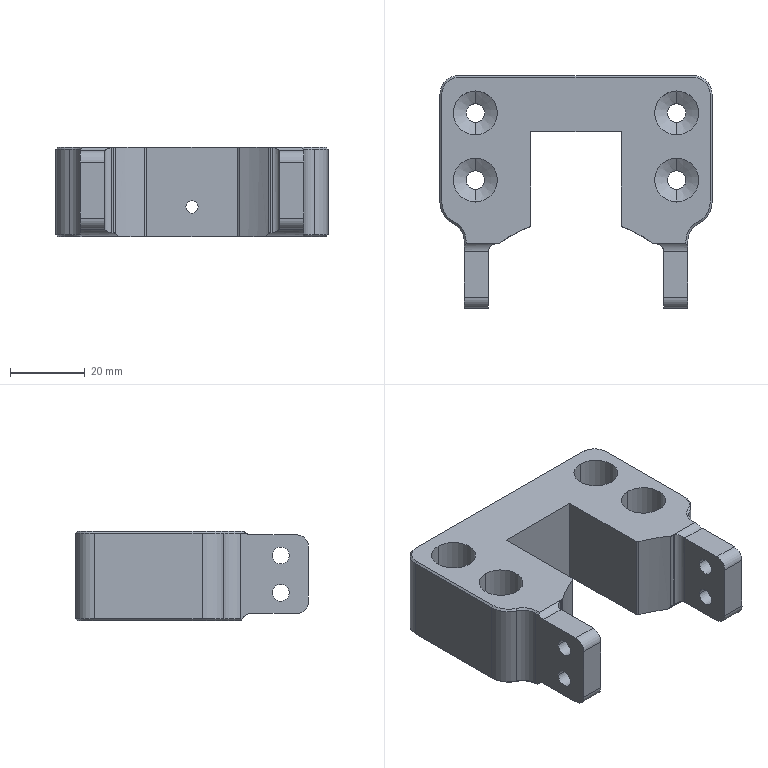NC program | NX | posted with a generic post | part box 73 x 62.4 x 24 mm
Lines 2249 to 2496 of 2496:
(ZLEVEL_PROFILE_1_COPY_1_COPY_COPY_1_COPY_COPY , TOOL : D6A45)
N4454 T07 M6
N4456 G54
N4458 G17 G0 G90 X27.544 Y21.2 S7500 M3
N4460 G43 Z30. H7
N4462 Z1.
N4464 G94 G1 Z-2. F1000.
N4466 G3 X26.999 Y21.744 R0.544
N4468 X27.544 Y21.2 R-0.544
N4470 X27.394 Y21.46 R0.3
N4472 G1 Z-1.
N4474 G0 Z30.
N4476 X-27.544 Y21.2
N4478 Z1.
N4480 G1 Z-2.
N4482 Y21.199
N4484 G3 X-26.999 Y20.656 R0.544
N4486 X-27.544 Y21.2 R-0.544
N4488 X-27.394 Y20.94 R0.3
N4490 G1 Z-1.
N4492 G0 Z30.
N4494 X27.544 Y3.2
N4496 Z1.
N4498 G1 Z-2.
N4500 G3 X27. Y3.744 R0.544
N4502 X27.544 Y3.2 R-0.544
N4504 X27.394 Y3.46 R0.3
N4506 G1 Z-1.
N4508 G0 Z30.
N4510 X-27.544 Y3.2
N4512 Z1.
N4514 G1 Z-2.
N4516 G3 X-27. Y2.656 R0.544
N4518 X-27.544 Y3.2 R-0.544
N4520 X-27.394 Y2.94 R0.3
N4522 G1 Z-1.
N4524 G0 Z30.
N4526 X-32.48 Y-14.397
N4528 Z-1.
N4530 G1 Z-2.
N4532 X-31.756 Y-13.979
N4534 G3 X-31.456 Y-13.459 R0.6
N4536 G1 Y-13.056
N4538 G3 X-33.459 Y-9.865 R3.544
N4540 G2 X-37.956 Y-2.7 R7.956
N4542 G1 Y26.2
N4544 G2 X-31.5 Y32.656 R6.456
N4546 G1 X31.5
N4548 G2 X37.956 Y26.2 R6.456
N4550 G1 Y-2.7
N4552 G2 X33.459 Y-9.865 R7.956
N4554 G3 X31.456 Y-13.056 R3.544
N4556 G1 Y-13.459
N4558 G3 X31.756 Y-13.979 R0.6
N4560 G1 X32.478 Y-14.395
N4562 Z-1.
N4564 G0 Z30.
N4566 X18.921 Y-16.249
N4568 Z-1.
N4570 G1 Z-2.
N4572 X18.987 Y-15.384
N4574 G3 X18.727 Y-14.843 R0.6
N4576 X11.937 Y-11.277 R33.194
N4578 G2 X10.346 Y-9.82 R2.956
N4580 X10.144 Y-8.955 R1.966
N4582 G1 Y14.244
N4584 X-10.144
N4586 Y-8.955
N4588 G2 X-10.339 Y-9.806 R1.954
N4590 X-11.937 Y-11.277 R2.956
N4592 G3 X-18.727 Y-14.843 R33.194
N4594 X-18.987 Y-15.384 R0.6
N4596 G1 X-18.921 Y-16.249
N4598 Z-1.
N4600 G0 Z30.
(ZLEVEL_PROFILE_1_COPY_1_COPY_COPY_1_COPY_COPY_COPY , TOOL : D6A45)
N4602 X21.438 Y-29.185
N4604 Z-2.
N4606 G1 Z-3.
N4608 X22.241 Y-28.721
N4610 G3 X22.541 Y-28.201 R0.6
N4612 G1 Y-16.42
N4614 G3 X22.022 Y-16.72 R0.6
N4616 G1 X21.341 Y-17.899
N4618 Z-2.
N4620 G0 Z30.
N4622 X32.159 Y-16.553
N4624 Z-2.
N4626 G1 Z-3.
N4628 X30.999 Y-16.007
N4630 X30.967 Y-16.051
N4632 X30.953 Y-16.103
N4634 X30.959 Y-16.157
N4636 Y-28.202
N4638 G3 X31.259 Y-28.721 R0.6
N4640 G1 X32.063 Y-29.186
N4642 Z-2.
N4644 G0 Z30.
N4646 X-32.062 Y-29.185
N4648 Z-2.
N4650 G1 Z-3.
N4652 X-31.259 Y-28.721
N4654 G3 X-30.959 Y-28.201 R0.6
N4656 G1 Y-16.158
N4658 X-30.953 Y-16.104
N4660 X-30.967 Y-16.052
N4662 X-30.999 Y-16.008
N4664 X-32.159 Y-16.552
N4666 Z-2.
N4668 G0 Z30.
N4670 X-21.341 Y-17.899
N4672 Z-2.
N4674 G1 Z-3.
N4676 X-22.022 Y-16.72
N4678 G3 X-22.541 Y-16.42 R0.6
N4680 G1 Y-28.202
N4682 G3 X-22.241 Y-28.721 R0.6
N4684 G1 X-21.437 Y-29.186
N4686 Z-2.
N4688 G0 Z30.
(ZLEVEL_PROFILE_1_COPY_1_COPY_COPY_1_COPY_COPY_COPY_1 , TOOL : D6A45)
N4690 G55
N4692 X27.544 Y21.2
N4694 Z1.
N4696 G1 Z-2.
N4698 G3 X26.999 Y21.744 R0.544
N4700 X27.544 Y21.2 R-0.544
N4702 X27.394 Y21.46 R0.3
N4704 G1 Z-1.
N4706 G0 Z30.
N4708 X-27.544 Y21.2
N4710 Z1.
N4712 G1 Z-2.
N4714 Y21.199
N4716 G3 X-26.999 Y20.656 R0.544
N4718 X-27.544 Y21.2 R-0.544
N4720 X-27.394 Y20.94 R0.3
N4722 G1 Z-1.
N4724 G0 Z30.
N4726 X27.544 Y3.2
N4728 Z1.
N4730 G1 Z-2.
N4732 G3 X27. Y3.744 R0.544
N4734 X27.544 Y3.2 R-0.544
N4736 X27.394 Y3.46 R0.3
N4738 G1 Z-1.
N4740 G0 Z30.
N4742 X-27.544 Y3.2
N4744 Z1.
N4746 G1 Z-2.
N4748 G3 X-27. Y2.656 R0.544
N4750 X-27.544 Y3.2 R-0.544
N4752 X-27.394 Y2.94 R0.3
N4754 G1 Z-1.
N4756 G0 Z30.
N4758 X-32.48 Y-14.397
N4760 Z-1.
N4762 G1 Z-2.
N4764 X-31.756 Y-13.979
N4766 G3 X-31.456 Y-13.459 R0.6
N4768 G1 Y-13.056
N4770 G3 X-33.459 Y-9.865 R3.544
N4772 G2 X-37.956 Y-2.7 R7.956
N4774 G1 Y26.2
N4776 G2 X-31.5 Y32.656 R6.456
N4778 G1 X31.5
N4780 G2 X37.956 Y26.2 R6.456
N4782 G1 Y-2.7
N4784 G2 X33.459 Y-9.865 R7.956
N4786 G3 X31.456 Y-13.056 R3.544
N4788 G1 Y-13.459
N4790 G3 X31.756 Y-13.979 R0.6
N4792 G1 X32.478 Y-14.395
N4794 Z-1.
N4796 G0 Z30.
N4798 X18.921 Y-16.249
N4800 Z-1.
N4802 G1 Z-2.
N4804 X18.987 Y-15.384
N4806 G3 X18.727 Y-14.843 R0.6
N4808 X11.937 Y-11.277 R33.194
N4810 G2 X10.346 Y-9.82 R2.956
N4812 X10.144 Y-8.955 R1.966
N4814 G1 Y14.244
N4816 X-10.144
N4818 Y-8.955
N4820 G2 X-10.339 Y-9.806 R1.954
N4822 X-11.937 Y-11.277 R2.956
N4824 G3 X-18.727 Y-14.843 R33.194
N4826 X-18.987 Y-15.384 R0.6
N4828 G1 X-18.921 Y-16.249
N4830 Z-1.
N4832 G0 Z30.
(ZLEVEL_PROFILE_1_COPY_1_COPY_COPY_1_COPY_COPY_COPY_COPY , TOOL : D6A45)
N4834 X21.438 Y-29.185
N4836 Z-2.
N4838 G1 Z-3.
N4840 X22.241 Y-28.721
N4842 G3 X22.541 Y-28.201 R0.6
N4844 G1 Y-16.42
N4846 G3 X22.022 Y-16.72 R0.6
N4848 G1 X21.341 Y-17.899
N4850 Z-2.
N4852 G0 Z30.
N4854 X32.159 Y-16.553
N4856 Z-2.
N4858 G1 Z-3.
N4860 X30.999 Y-16.007
N4862 X30.967 Y-16.051
N4864 X30.953 Y-16.103
N4866 X30.959 Y-16.157
N4868 Y-28.202
N4870 G3 X31.259 Y-28.721 R0.6
N4872 G1 X32.063 Y-29.186
N4874 Z-2.
N4876 G0 Z30.
N4878 X-32.062 Y-29.185
N4880 Z-2.
N4882 G1 Z-3.
N4884 X-31.259 Y-28.721
N4886 G3 X-30.959 Y-28.201 R0.6
N4888 G1 Y-16.158
N4890 X-30.953 Y-16.104
N4892 X-30.967 Y-16.052
N4894 X-30.999 Y-16.008
N4896 X-32.159 Y-16.552
N4898 Z-2.
N4900 G0 Z30.
N4902 X-21.341 Y-17.899
N4904 Z-2.
N4906 G1 Z-3.
N4908 X-22.022 Y-16.72
N4910 G3 X-22.541 Y-16.42 R0.6
N4912 G1 Y-28.202
N4914 G3 X-22.241 Y-28.721 R0.6
N4916 G1 X-21.437 Y-29.186
N4918 Z-2.
N4920 G0 Z30.
N4922 M5
N4924 M2